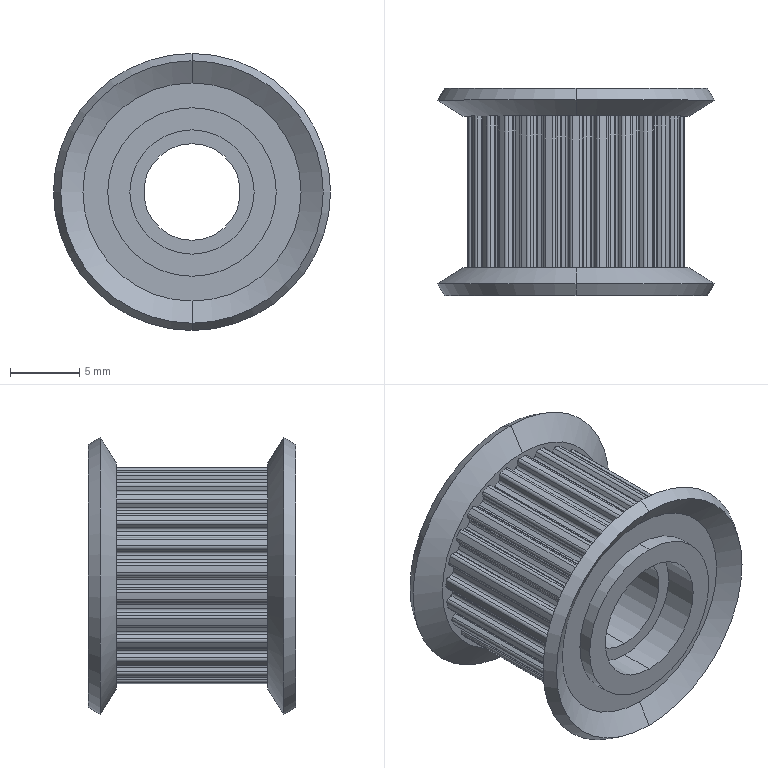Part | NX | features BREP 1 | 1 solid | 250 faces | box 20.061 x 15 x 20.061 mm | volume 2125 mm3 | cylinder 155 | plane 83 | cone 12 | commonest cylinder face diameters 0.46 x120 15.66 x25 9 x4 12.2 x4 7 x2